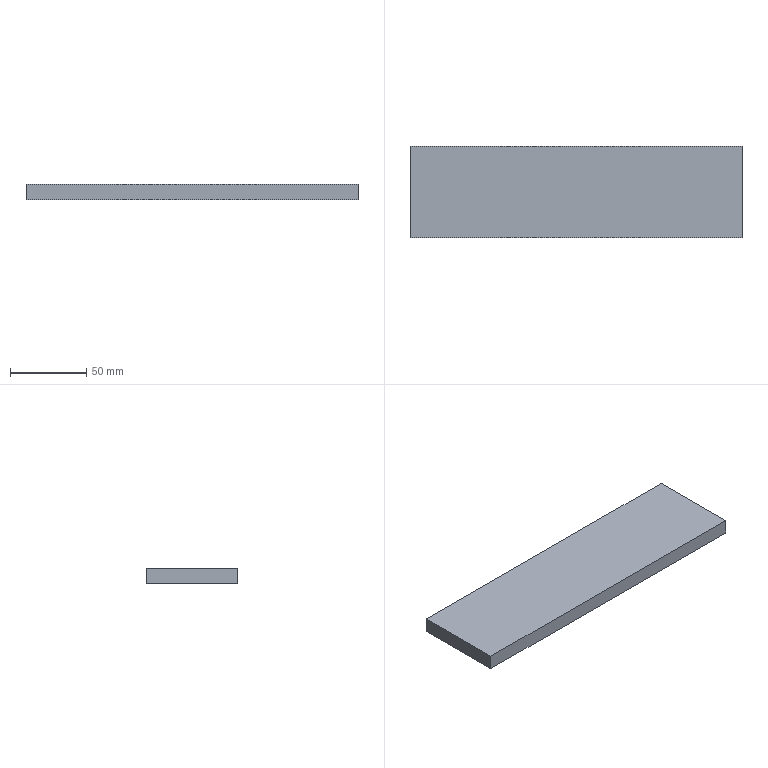Part | SolidWorks | features Extrusion 1 | 1 solid | 6 faces | box 218.3 x 60 x 10 mm | volume 130980 mm3 | plane 6
STEP:
#1=CARTESIAN_POINT('',(-109.15,30.,0.));
#2=VERTEX_POINT('',#1);
#3=CARTESIAN_POINT('',(-109.15,-30.,0.));
#4=VERTEX_POINT('',#3);
#5=CARTESIAN_POINT('',(-109.15,30.,0.));
#6=DIRECTION('',(0.,-1.,0.));
#7=VECTOR('',#6,1000.);
#8=LINE('',#5,#7);
#9=EDGE_CURVE('',#2,#4,#8,.T.);
#10=ORIENTED_EDGE('',*,*,#9,.T.);
#11=CARTESIAN_POINT('',(-109.15,-30.,10.));
#12=VERTEX_POINT('',#11);
#13=CARTESIAN_POINT('',(-109.15,-30.,10.));
#14=DIRECTION('',(0.,0.,-1.));
#15=VECTOR('',#14,1000.);
#16=LINE('',#13,#15);
#17=EDGE_CURVE('',#12,#4,#16,.T.);
#18=ORIENTED_EDGE('',*,*,#17,.F.);
#19=CARTESIAN_POINT('',(-109.15,30.,10.));
#20=VERTEX_POINT('',#19);
#21=CARTESIAN_POINT('',(-109.15,30.,10.));
#22=DIRECTION('',(0.,-1.,0.));
#23=VECTOR('',#22,1000.);
#24=LINE('',#21,#23);
#25=EDGE_CURVE('',#20,#12,#24,.T.);
#26=ORIENTED_EDGE('',*,*,#25,.F.);
#27=CARTESIAN_POINT('',(-109.15,30.,10.));
#28=DIRECTION('',(0.,0.,-1.));
#29=VECTOR('',#28,1000.);
#30=LINE('',#27,#29);
#31=EDGE_CURVE('',#20,#2,#30,.T.);
#32=ORIENTED_EDGE('',*,*,#31,.T.);
#33=EDGE_LOOP('',(#10,#18,#26,#32));
#34=FACE_OUTER_BOUND('',#33,.T.);
#35=CARTESIAN_POINT('',(-109.15,30.,10.));
#36=DIRECTION('',(1.,0.,0.));
#37=DIRECTION('',(0.,1.,0.));
#38=AXIS2_PLACEMENT_3D('',#35,#36,#37);
#39=PLANE('',#38);
#40=ADVANCED_FACE('',(#34),#39,.F.);
#41=CARTESIAN_POINT('',(109.15,-30.,0.));
#42=VERTEX_POINT('',#41);
#43=CARTESIAN_POINT('',(109.15,-30.,0.));
#44=DIRECTION('',(1.,0.,0.));
#45=VECTOR('',#44,1000.);
#46=LINE('',#43,#45);
#47=EDGE_CURVE('',#4,#42,#46,.T.);
#48=ORIENTED_EDGE('',*,*,#47,.T.);
#49=CARTESIAN_POINT('',(109.15,-30.,10.));
#50=VERTEX_POINT('',#49);
#51=CARTESIAN_POINT('',(109.15,-30.,10.));
#52=DIRECTION('',(0.,0.,-1.));
#53=VECTOR('',#52,1000.);
#54=LINE('',#51,#53);
#55=EDGE_CURVE('',#50,#42,#54,.T.);
#56=ORIENTED_EDGE('',*,*,#55,.F.);
#57=CARTESIAN_POINT('',(109.15,-30.,10.));
#58=DIRECTION('',(1.,0.,0.));
#59=VECTOR('',#58,1000.);
#60=LINE('',#57,#59);
#61=EDGE_CURVE('',#12,#50,#60,.T.);
#62=ORIENTED_EDGE('',*,*,#61,.F.);
#63=ORIENTED_EDGE('',*,*,#17,.T.);
#64=EDGE_LOOP('',(#48,#56,#62,#63));
#65=FACE_OUTER_BOUND('',#64,.T.);
#66=CARTESIAN_POINT('',(109.15,-30.,10.));
#67=DIRECTION('',(0.,1.,0.));
#68=DIRECTION('',(-1.,0.,0.));
#69=AXIS2_PLACEMENT_3D('',#66,#67,#68);
#70=PLANE('',#69);
#71=ADVANCED_FACE('',(#65),#70,.F.);
#72=CARTESIAN_POINT('',(109.15,30.,0.));
#73=VERTEX_POINT('',#72);
#74=CARTESIAN_POINT('',(109.15,30.,0.));
#75=DIRECTION('',(0.,1.,0.));
#76=VECTOR('',#75,1000.);
#77=LINE('',#74,#76);
#78=EDGE_CURVE('',#42,#73,#77,.T.);
#79=ORIENTED_EDGE('',*,*,#78,.T.);
#80=CARTESIAN_POINT('',(109.15,30.,10.));
#81=VERTEX_POINT('',#80);
#82=CARTESIAN_POINT('',(109.15,30.,10.));
#83=DIRECTION('',(0.,0.,-1.));
#84=VECTOR('',#83,1000.);
#85=LINE('',#82,#84);
#86=EDGE_CURVE('',#81,#73,#85,.T.);
#87=ORIENTED_EDGE('',*,*,#86,.F.);
#88=CARTESIAN_POINT('',(109.15,30.,10.));
#89=DIRECTION('',(0.,1.,0.));
#90=VECTOR('',#89,1000.);
#91=LINE('',#88,#90);
#92=EDGE_CURVE('',#50,#81,#91,.T.);
#93=ORIENTED_EDGE('',*,*,#92,.F.);
#94=ORIENTED_EDGE('',*,*,#55,.T.);
#95=EDGE_LOOP('',(#79,#87,#93,#94));
#96=FACE_OUTER_BOUND('',#95,.T.);
#97=CARTESIAN_POINT('',(109.15,30.,10.));
#98=DIRECTION('',(-1.,0.,0.));
#99=DIRECTION('',(0.,-1.,0.));
#100=AXIS2_PLACEMENT_3D('',#97,#98,#99);
#101=PLANE('',#100);
#102=ADVANCED_FACE('',(#96),#101,.F.);
#103=CARTESIAN_POINT('',(109.15,30.,0.));
#104=DIRECTION('',(-1.,0.,0.));
#105=VECTOR('',#104,1000.);
#106=LINE('',#103,#105);
#107=EDGE_CURVE('',#73,#2,#106,.T.);
#108=ORIENTED_EDGE('',*,*,#107,.T.);
#109=ORIENTED_EDGE('',*,*,#31,.F.);
#110=CARTESIAN_POINT('',(109.15,30.,10.));
#111=DIRECTION('',(-1.,0.,0.));
#112=VECTOR('',#111,1000.);
#113=LINE('',#110,#112);
#114=EDGE_CURVE('',#81,#20,#113,.T.);
#115=ORIENTED_EDGE('',*,*,#114,.F.);
#116=ORIENTED_EDGE('',*,*,#86,.T.);
#117=EDGE_LOOP('',(#108,#109,#115,#116));
#118=FACE_OUTER_BOUND('',#117,.T.);
#119=CARTESIAN_POINT('',(109.15,30.,10.));
#120=DIRECTION('',(0.,-1.,0.));
#121=DIRECTION('',(1.,0.,0.));
#122=AXIS2_PLACEMENT_3D('',#119,#120,#121);
#123=PLANE('',#122);
#124=ADVANCED_FACE('',(#118),#123,.F.);
#125=ORIENTED_EDGE('',*,*,#25,.T.);
#126=ORIENTED_EDGE('',*,*,#61,.T.);
#127=ORIENTED_EDGE('',*,*,#92,.T.);
#128=ORIENTED_EDGE('',*,*,#114,.T.);
#129=EDGE_LOOP('',(#125,#126,#127,#128));
#130=FACE_OUTER_BOUND('',#129,.T.);
#131=CARTESIAN_POINT('',(0.,0.,10.));
#132=DIRECTION('',(0.,0.,-1.));
#133=DIRECTION('',(-1.,0.,0.));
#134=AXIS2_PLACEMENT_3D('',#131,#132,#133);
#135=PLANE('',#134);
#136=ADVANCED_FACE('',(#130),#135,.F.);
#137=ORIENTED_EDGE('',*,*,#9,.F.);
#138=ORIENTED_EDGE('',*,*,#107,.F.);
#139=ORIENTED_EDGE('',*,*,#78,.F.);
#140=ORIENTED_EDGE('',*,*,#47,.F.);
#141=EDGE_LOOP('',(#137,#138,#139,#140));
#142=FACE_OUTER_BOUND('',#141,.T.);
#143=CARTESIAN_POINT('',(0.,0.,0.));
#144=DIRECTION('',(0.,0.,-1.));
#145=DIRECTION('',(-1.,0.,0.));
#146=AXIS2_PLACEMENT_3D('',#143,#144,#145);
#147=PLANE('',#146);
#148=ADVANCED_FACE('',(#142),#147,.T.);
#149=CLOSED_SHELL('',(#40,#71,#102,#124,#136,#148));
#150=MANIFOLD_SOLID_BREP('',#149);
#151=CARTESIAN_POINT('',(0.,0.,0.));
#152=DIRECTION('',(0.,0.,1.));
#153=DIRECTION('',(1.,0.,0.));
#154=AXIS2_PLACEMENT_3D('',#151,#152,#153);
#155=(LENGTH_UNIT()NAMED_UNIT(*)SI_UNIT(.MILLI.,.METRE.));
#156=UNCERTAINTY_MEASURE_WITH_UNIT(LENGTH_MEASURE(0.00001),#155,'','');
#157=(NAMED_UNIT(*)PLANE_ANGLE_UNIT()SI_UNIT($,.RADIAN.));
#158=(NAMED_UNIT(*)SI_UNIT($,.STERADIAN.)SOLID_ANGLE_UNIT());
#159=(GEOMETRIC_REPRESENTATION_CONTEXT(3)GLOBAL_UNCERTAINTY_ASSIGNED_CONTEXT((#156))GLOBAL_UNIT_ASSIGNED_CONTEXT((#155,#157,#158))REPRESENTATION_CONTEXT('',''));
#160=ADVANCED_BREP_SHAPE_REPRESENTATION('',(#150,#154),#159);